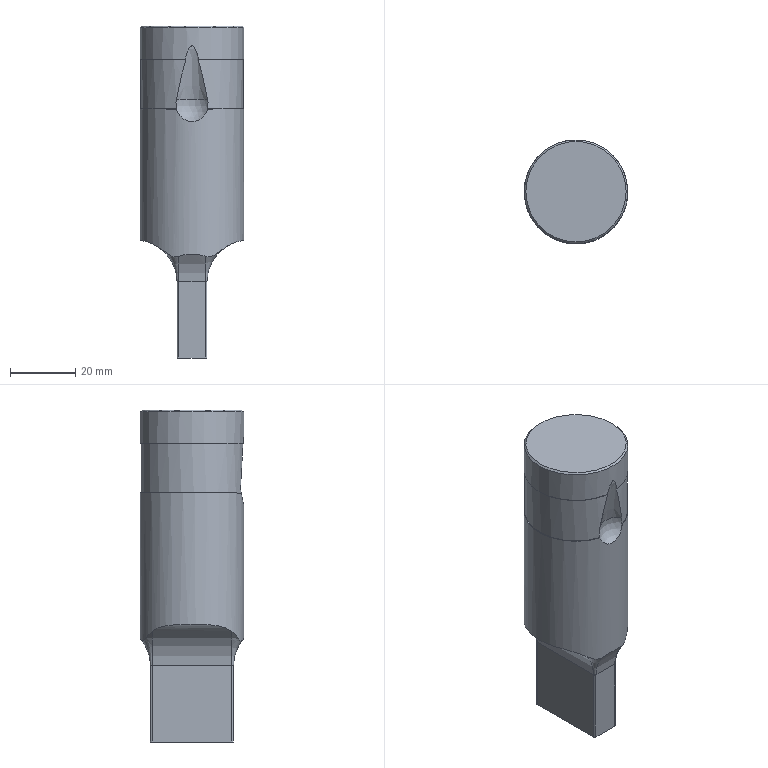Part | STEP file | 1_id654_x_t | 1 solid | 26 faces | box 31.75 x 31.75 x 101.6 mm | volume 61988 mm3 | cylinder 11 | plane 8 | torus 4 | cone 2 | sphere 1 | commonest cylinder face diameters 1.016 x4 25.4 x4 31.75 x2 31.344 x1